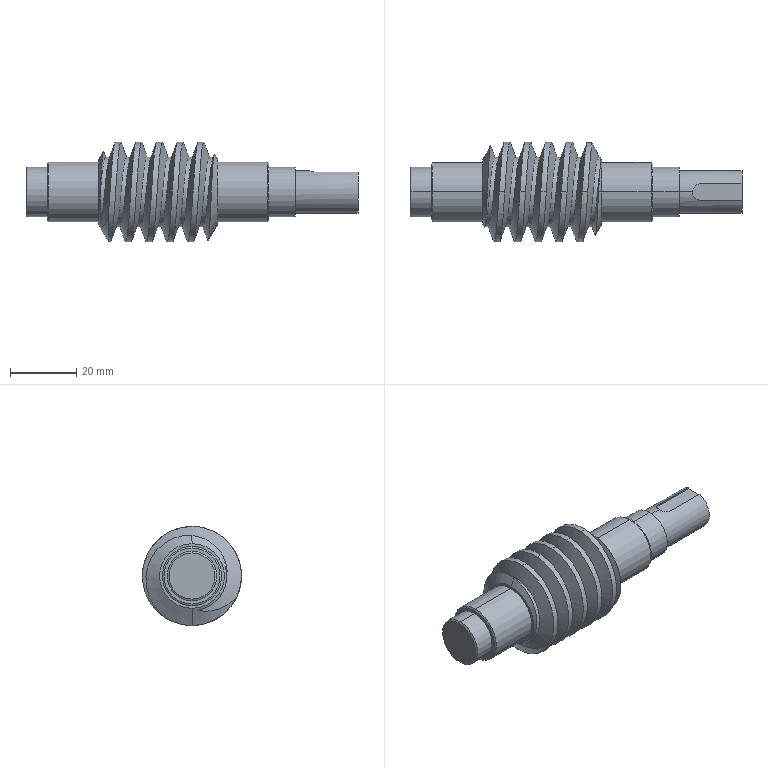Part | SolidWorks | features ICE 6, Chamfer 1, Extrusion 1, Helix 1, RevCut 1, SweepCut 1 | 1 solid | 45 faces | box 100.5 x 30 x 30 mm | volume 31439 mm3 | cylinder 22 | cone 10 | plane 10 | spline 3 | commonest cylinder face diameters 30 x11 15 x4 18 x4 13 x2 5 x1